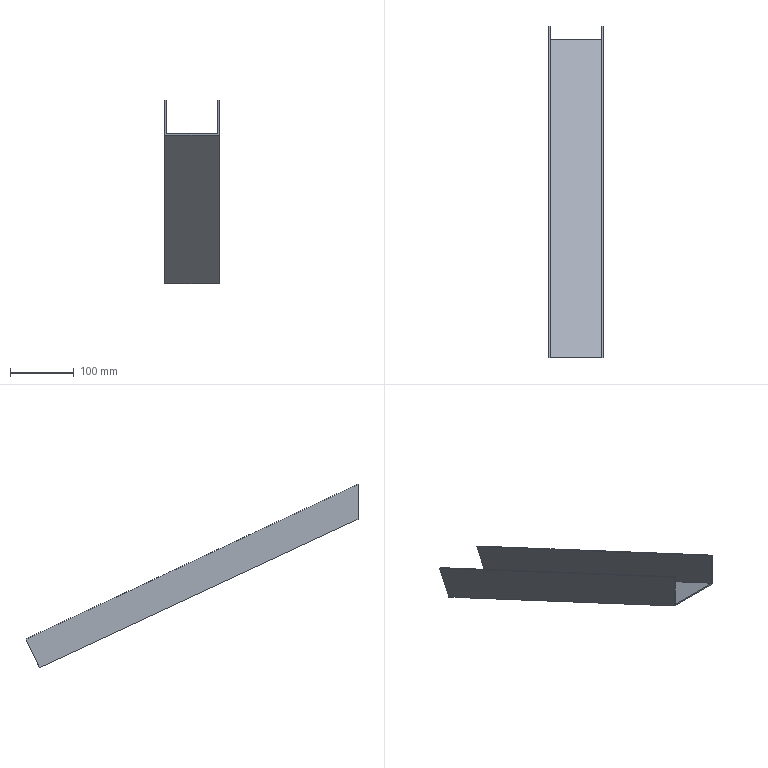Part | NX | features solid 2 | 1 solid | 10 faces | box 85 x 521.131 x 288.323 mm | volume 202118 mm3 | plane 10
STEP:
#1=CARTESIAN_POINT('',(400.,525.,-154.948));
#2=VERTEX_POINT('',#1);
#3=CARTESIAN_POINT('',(402.,525.,-154.948));
#4=VERTEX_POINT('',#3);
#5=CARTESIAN_POINT('',(400.,525.,-154.948));
#6=DIRECTION('',(1.,0.,0.));
#7=VECTOR('',#6,1000.);
#8=LINE('',#5,#7);
#9=EDGE_CURVE('',#2,#4,#8,.T.);
#10=ORIENTED_EDGE('',*,*,#9,.F.);
#11=CARTESIAN_POINT('',(400.,525.,-210.116));
#12=VERTEX_POINT('',#11);
#13=CARTESIAN_POINT('',(400.,525.,-175.106));
#14=DIRECTION('',(0.,0.,-1.));
#15=VECTOR('',#14,1000.);
#16=LINE('',#13,#15);
#17=EDGE_CURVE('',#2,#12,#16,.T.);
#18=ORIENTED_EDGE('',*,*,#17,.T.);
#19=CARTESIAN_POINT('',(485.,525.,-210.116));
#20=VERTEX_POINT('',#19);
#21=CARTESIAN_POINT('',(400.,525.,-210.116));
#22=DIRECTION('',(1.,0.,0.));
#23=VECTOR('',#22,1000.);
#24=LINE('',#21,#23);
#25=EDGE_CURVE('',#12,#20,#24,.T.);
#26=ORIENTED_EDGE('',*,*,#25,.T.);
#27=CARTESIAN_POINT('',(485.,525.,-154.948));
#28=VERTEX_POINT('',#27);
#29=CARTESIAN_POINT('',(485.,525.,-175.106));
#30=DIRECTION('',(0.,0.,-1.));
#31=VECTOR('',#30,1000.);
#32=LINE('',#29,#31);
#33=EDGE_CURVE('',#28,#20,#32,.T.);
#34=ORIENTED_EDGE('',*,*,#33,.F.);
#35=CARTESIAN_POINT('',(483.,525.,-154.948));
#36=VERTEX_POINT('',#35);
#37=CARTESIAN_POINT('',(400.,525.,-154.948));
#38=DIRECTION('',(1.,0.,0.));
#39=VECTOR('',#38,1000.);
#40=LINE('',#37,#39);
#41=EDGE_CURVE('',#36,#28,#40,.T.);
#42=ORIENTED_EDGE('',*,*,#41,.F.);
#43=CARTESIAN_POINT('',(483.,525.,-207.91));
#44=VERTEX_POINT('',#43);
#45=CARTESIAN_POINT('',(483.,525.,-175.106));
#46=DIRECTION('',(0.,0.,-1.));
#47=VECTOR('',#46,1000.);
#48=LINE('',#45,#47);
#49=EDGE_CURVE('',#36,#44,#48,.T.);
#50=ORIENTED_EDGE('',*,*,#49,.T.);
#51=CARTESIAN_POINT('',(402.,525.,-207.91));
#52=VERTEX_POINT('',#51);
#53=CARTESIAN_POINT('',(400.,525.,-207.91));
#54=DIRECTION('',(1.,0.,0.));
#55=VECTOR('',#54,1000.);
#56=LINE('',#53,#55);
#57=EDGE_CURVE('',#52,#44,#56,.T.);
#58=ORIENTED_EDGE('',*,*,#57,.F.);
#59=CARTESIAN_POINT('',(402.,525.,-175.106));
#60=DIRECTION('',(0.,0.,-1.));
#61=VECTOR('',#60,1000.);
#62=LINE('',#59,#61);
#63=EDGE_CURVE('',#4,#52,#62,.T.);
#64=ORIENTED_EDGE('',*,*,#63,.F.);
#65=EDGE_LOOP('',(#10,#18,#26,#34,#42,#50,#58,#64));
#66=FACE_BOUND('',#65,.T.);
#67=CARTESIAN_POINT('',(-1120.,525.,-215.));
#68=DIRECTION('',(0.,-1.,0.));
#69=DIRECTION('',(-1.,0.,0.));
#70=AXIS2_PLACEMENT_3D('',#67,#68,#69);
#71=PLANE('',#70);
#72=ADVANCED_FACE('',(#66),#71,.T.);
#73=CARTESIAN_POINT('',(485.,1046.131,-397.955));
#74=VERTEX_POINT('',#73);
#75=CARTESIAN_POINT('',(483.,1046.131,-397.955));
#76=VERTEX_POINT('',#75);
#77=CARTESIAN_POINT('',(400.,1046.131,-397.955));
#78=DIRECTION('',(-1.,0.,0.));
#79=VECTOR('',#78,1000.);
#80=LINE('',#77,#79);
#81=EDGE_CURVE('',#74,#76,#80,.T.);
#82=ORIENTED_EDGE('',*,*,#81,.F.);
#83=CARTESIAN_POINT('',(485.,1025.,-443.27));
#84=VERTEX_POINT('',#83);
#85=CARTESIAN_POINT('',(485.,1046.131,-397.955));
#86=DIRECTION('',(0.,-0.4226,-0.9063));
#87=VECTOR('',#86,1000.);
#88=LINE('',#85,#87);
#89=EDGE_CURVE('',#74,#84,#88,.T.);
#90=ORIENTED_EDGE('',*,*,#89,.T.);
#91=CARTESIAN_POINT('',(400.,1025.,-443.27));
#92=VERTEX_POINT('',#91);
#93=CARTESIAN_POINT('',(400.,1025.,-443.27));
#94=DIRECTION('',(-1.,0.,0.));
#95=VECTOR('',#94,1000.);
#96=LINE('',#93,#95);
#97=EDGE_CURVE('',#84,#92,#96,.T.);
#98=ORIENTED_EDGE('',*,*,#97,.T.);
#99=CARTESIAN_POINT('',(400.,1046.131,-397.955));
#100=VERTEX_POINT('',#99);
#101=CARTESIAN_POINT('',(400.,1046.131,-397.955));
#102=DIRECTION('',(0.,-0.4226,-0.9063));
#103=VECTOR('',#102,1000.);
#104=LINE('',#101,#103);
#105=EDGE_CURVE('',#100,#92,#104,.T.);
#106=ORIENTED_EDGE('',*,*,#105,.F.);
#107=CARTESIAN_POINT('',(402.,1046.131,-397.955));
#108=VERTEX_POINT('',#107);
#109=CARTESIAN_POINT('',(400.,1046.131,-397.955));
#110=DIRECTION('',(-1.,0.,0.));
#111=VECTOR('',#110,1000.);
#112=LINE('',#109,#111);
#113=EDGE_CURVE('',#108,#100,#112,.T.);
#114=ORIENTED_EDGE('',*,*,#113,.F.);
#115=CARTESIAN_POINT('',(402.,1025.845,-441.458));
#116=VERTEX_POINT('',#115);
#117=CARTESIAN_POINT('',(402.,1046.131,-397.955));
#118=DIRECTION('',(0.,-0.4226,-0.9063));
#119=VECTOR('',#118,1000.);
#120=LINE('',#117,#119);
#121=EDGE_CURVE('',#108,#116,#120,.T.);
#122=ORIENTED_EDGE('',*,*,#121,.T.);
#123=CARTESIAN_POINT('',(483.,1025.845,-441.458));
#124=VERTEX_POINT('',#123);
#125=CARTESIAN_POINT('',(400.,1025.845,-441.458));
#126=DIRECTION('',(-1.,0.,0.));
#127=VECTOR('',#126,1000.);
#128=LINE('',#125,#127);
#129=EDGE_CURVE('',#124,#116,#128,.T.);
#130=ORIENTED_EDGE('',*,*,#129,.F.);
#131=CARTESIAN_POINT('',(483.,1046.131,-397.955));
#132=DIRECTION('',(0.,-0.4226,-0.9063));
#133=VECTOR('',#132,1000.);
#134=LINE('',#131,#133);
#135=EDGE_CURVE('',#76,#124,#134,.T.);
#136=ORIENTED_EDGE('',*,*,#135,.F.);
#137=EDGE_LOOP('',(#82,#90,#98,#106,#114,#122,#130,#136));
#138=FACE_BOUND('',#137,.T.);
#139=CARTESIAN_POINT('',(400.,1046.131,-397.955));
#140=DIRECTION('',(0.,0.9063,-0.4226));
#141=DIRECTION('',(0.,-0.4226,-0.9063));
#142=AXIS2_PLACEMENT_3D('',#139,#140,#141);
#143=PLANE('',#142);
#144=ADVANCED_FACE('',(#138),#143,.T.);
#145=ORIENTED_EDGE('',*,*,#113,.T.);
#146=CARTESIAN_POINT('',(400.,568.231,-175.106));
#147=DIRECTION('',(0.,-0.9063,0.4226));
#148=VECTOR('',#147,1000.);
#149=LINE('',#146,#148);
#150=EDGE_CURVE('',#100,#2,#149,.T.);
#151=ORIENTED_EDGE('',*,*,#150,.T.);
#152=ORIENTED_EDGE('',*,*,#9,.T.);
#153=CARTESIAN_POINT('',(402.,568.231,-175.106));
#154=DIRECTION('',(0.,-0.9063,0.4226));
#155=VECTOR('',#154,1000.);
#156=LINE('',#153,#155);
#157=EDGE_CURVE('',#108,#4,#156,.T.);
#158=ORIENTED_EDGE('',*,*,#157,.F.);
#159=EDGE_LOOP('',(#145,#151,#152,#158));
#160=FACE_BOUND('',#159,.T.);
#161=CARTESIAN_POINT('',(400.,568.231,-175.106));
#162=DIRECTION('',(0.,-0.4226,-0.9063));
#163=DIRECTION('',(-1.,0.,0.));
#164=AXIS2_PLACEMENT_3D('',#161,#162,#163);
#165=PLANE('',#164);
#166=ADVANCED_FACE('',(#160),#165,.F.);
#167=CARTESIAN_POINT('',(400.,547.1,-220.422));
#168=DIRECTION('',(0.,-0.9063,0.4226));
#169=VECTOR('',#168,1000.);
#170=LINE('',#167,#169);
#171=EDGE_CURVE('',#92,#12,#170,.T.);
#172=ORIENTED_EDGE('',*,*,#171,.T.);
#173=ORIENTED_EDGE('',*,*,#17,.F.);
#174=ORIENTED_EDGE('',*,*,#150,.F.);
#175=ORIENTED_EDGE('',*,*,#105,.T.);
#176=EDGE_LOOP('',(#172,#173,#174,#175));
#177=FACE_BOUND('',#176,.T.);
#178=CARTESIAN_POINT('',(400.,568.231,-175.106));
#179=DIRECTION('',(-1.,0.,0.));
#180=DIRECTION('',(0.,0.,1.));
#181=AXIS2_PLACEMENT_3D('',#178,#179,#180);
#182=PLANE('',#181);
#183=ADVANCED_FACE('',(#177),#182,.T.);
#184=CARTESIAN_POINT('',(485.,547.1,-220.422));
#185=DIRECTION('',(0.,0.9063,-0.4226));
#186=VECTOR('',#185,1000.);
#187=LINE('',#184,#186);
#188=EDGE_CURVE('',#20,#84,#187,.T.);
#189=ORIENTED_EDGE('',*,*,#188,.T.);
#190=ORIENTED_EDGE('',*,*,#89,.F.);
#191=CARTESIAN_POINT('',(485.,568.231,-175.106));
#192=DIRECTION('',(0.,0.9063,-0.4226));
#193=VECTOR('',#192,1000.);
#194=LINE('',#191,#193);
#195=EDGE_CURVE('',#28,#74,#194,.T.);
#196=ORIENTED_EDGE('',*,*,#195,.F.);
#197=ORIENTED_EDGE('',*,*,#33,.T.);
#198=EDGE_LOOP('',(#189,#190,#196,#197));
#199=FACE_BOUND('',#198,.T.);
#200=CARTESIAN_POINT('',(485.,568.231,-175.106));
#201=DIRECTION('',(1.,0.,0.));
#202=DIRECTION('',(0.,0.,-1.));
#203=AXIS2_PLACEMENT_3D('',#200,#201,#202);
#204=PLANE('',#203);
#205=ADVANCED_FACE('',(#199),#204,.T.);
#206=ORIENTED_EDGE('',*,*,#41,.T.);
#207=ORIENTED_EDGE('',*,*,#195,.T.);
#208=ORIENTED_EDGE('',*,*,#81,.T.);
#209=CARTESIAN_POINT('',(483.,568.231,-175.106));
#210=DIRECTION('',(0.,0.9063,-0.4226));
#211=VECTOR('',#210,1000.);
#212=LINE('',#209,#211);
#213=EDGE_CURVE('',#36,#76,#212,.T.);
#214=ORIENTED_EDGE('',*,*,#213,.F.);
#215=EDGE_LOOP('',(#206,#207,#208,#214));
#216=FACE_BOUND('',#215,.T.);
#217=CARTESIAN_POINT('',(400.,568.231,-175.106));
#218=DIRECTION('',(0.,-0.4226,-0.9063));
#219=DIRECTION('',(-1.,0.,0.));
#220=AXIS2_PLACEMENT_3D('',#217,#218,#219);
#221=PLANE('',#220);
#222=ADVANCED_FACE('',(#216),#221,.F.);
#223=ORIENTED_EDGE('',*,*,#171,.F.);
#224=ORIENTED_EDGE('',*,*,#97,.F.);
#225=ORIENTED_EDGE('',*,*,#188,.F.);
#226=ORIENTED_EDGE('',*,*,#25,.F.);
#227=EDGE_LOOP('',(#223,#224,#225,#226));
#228=FACE_BOUND('',#227,.T.);
#229=CARTESIAN_POINT('',(400.,547.1,-220.422));
#230=DIRECTION('',(0.,-0.4226,-0.9063));
#231=DIRECTION('',(-1.,0.,0.));
#232=AXIS2_PLACEMENT_3D('',#229,#230,#231);
#233=PLANE('',#232);
#234=ADVANCED_FACE('',(#228),#233,.T.);
#235=CARTESIAN_POINT('',(402.,547.945,-218.609));
#236=DIRECTION('',(0.,-0.9063,0.4226));
#237=VECTOR('',#236,1000.);
#238=LINE('',#235,#237);
#239=EDGE_CURVE('',#116,#52,#238,.T.);
#240=ORIENTED_EDGE('',*,*,#239,.F.);
#241=ORIENTED_EDGE('',*,*,#121,.F.);
#242=ORIENTED_EDGE('',*,*,#157,.T.);
#243=ORIENTED_EDGE('',*,*,#63,.T.);
#244=EDGE_LOOP('',(#240,#241,#242,#243));
#245=FACE_BOUND('',#244,.T.);
#246=CARTESIAN_POINT('',(402.,568.231,-175.106));
#247=DIRECTION('',(-1.,0.,0.));
#248=DIRECTION('',(0.,0.,1.));
#249=AXIS2_PLACEMENT_3D('',#246,#247,#248);
#250=PLANE('',#249);
#251=ADVANCED_FACE('',(#245),#250,.F.);
#252=CARTESIAN_POINT('',(483.,547.945,-218.609));
#253=DIRECTION('',(0.,0.9063,-0.4226));
#254=VECTOR('',#253,1000.);
#255=LINE('',#252,#254);
#256=EDGE_CURVE('',#44,#124,#255,.T.);
#257=ORIENTED_EDGE('',*,*,#256,.F.);
#258=ORIENTED_EDGE('',*,*,#49,.F.);
#259=ORIENTED_EDGE('',*,*,#213,.T.);
#260=ORIENTED_EDGE('',*,*,#135,.T.);
#261=EDGE_LOOP('',(#257,#258,#259,#260));
#262=FACE_BOUND('',#261,.T.);
#263=CARTESIAN_POINT('',(483.,568.231,-175.106));
#264=DIRECTION('',(1.,0.,0.));
#265=DIRECTION('',(0.,0.,-1.));
#266=AXIS2_PLACEMENT_3D('',#263,#264,#265);
#267=PLANE('',#266);
#268=ADVANCED_FACE('',(#262),#267,.F.);
#269=ORIENTED_EDGE('',*,*,#239,.T.);
#270=ORIENTED_EDGE('',*,*,#57,.T.);
#271=ORIENTED_EDGE('',*,*,#256,.T.);
#272=ORIENTED_EDGE('',*,*,#129,.T.);
#273=EDGE_LOOP('',(#269,#270,#271,#272));
#274=FACE_BOUND('',#273,.T.);
#275=CARTESIAN_POINT('',(400.,547.945,-218.609));
#276=DIRECTION('',(0.,-0.4226,-0.9063));
#277=DIRECTION('',(-1.,0.,0.));
#278=AXIS2_PLACEMENT_3D('',#275,#276,#277);
#279=PLANE('',#278);
#280=ADVANCED_FACE('',(#274),#279,.F.);
#281=CLOSED_SHELL('',(#72,#144,#166,#183,#205,#222,#234,#251,#268,#280));
#282=MANIFOLD_SOLID_BREP('',#281);
#283=(LENGTH_UNIT()NAMED_UNIT(*)SI_UNIT(.MILLI.,.METRE.));
#284=UNCERTAINTY_MEASURE_WITH_UNIT(LENGTH_MEASURE(0.00001),#283,'','');
#285=(NAMED_UNIT(*)PLANE_ANGLE_UNIT()SI_UNIT($,.RADIAN.));
#286=(NAMED_UNIT(*)SI_UNIT($,.STERADIAN.)SOLID_ANGLE_UNIT());
#287=(GEOMETRIC_REPRESENTATION_CONTEXT(3)GLOBAL_UNCERTAINTY_ASSIGNED_CONTEXT((#284))GLOBAL_UNIT_ASSIGNED_CONTEXT((#283,#285,#286))REPRESENTATION_CONTEXT('',''));
#288=ADVANCED_BREP_SHAPE_REPRESENTATION('',(#282),#287);